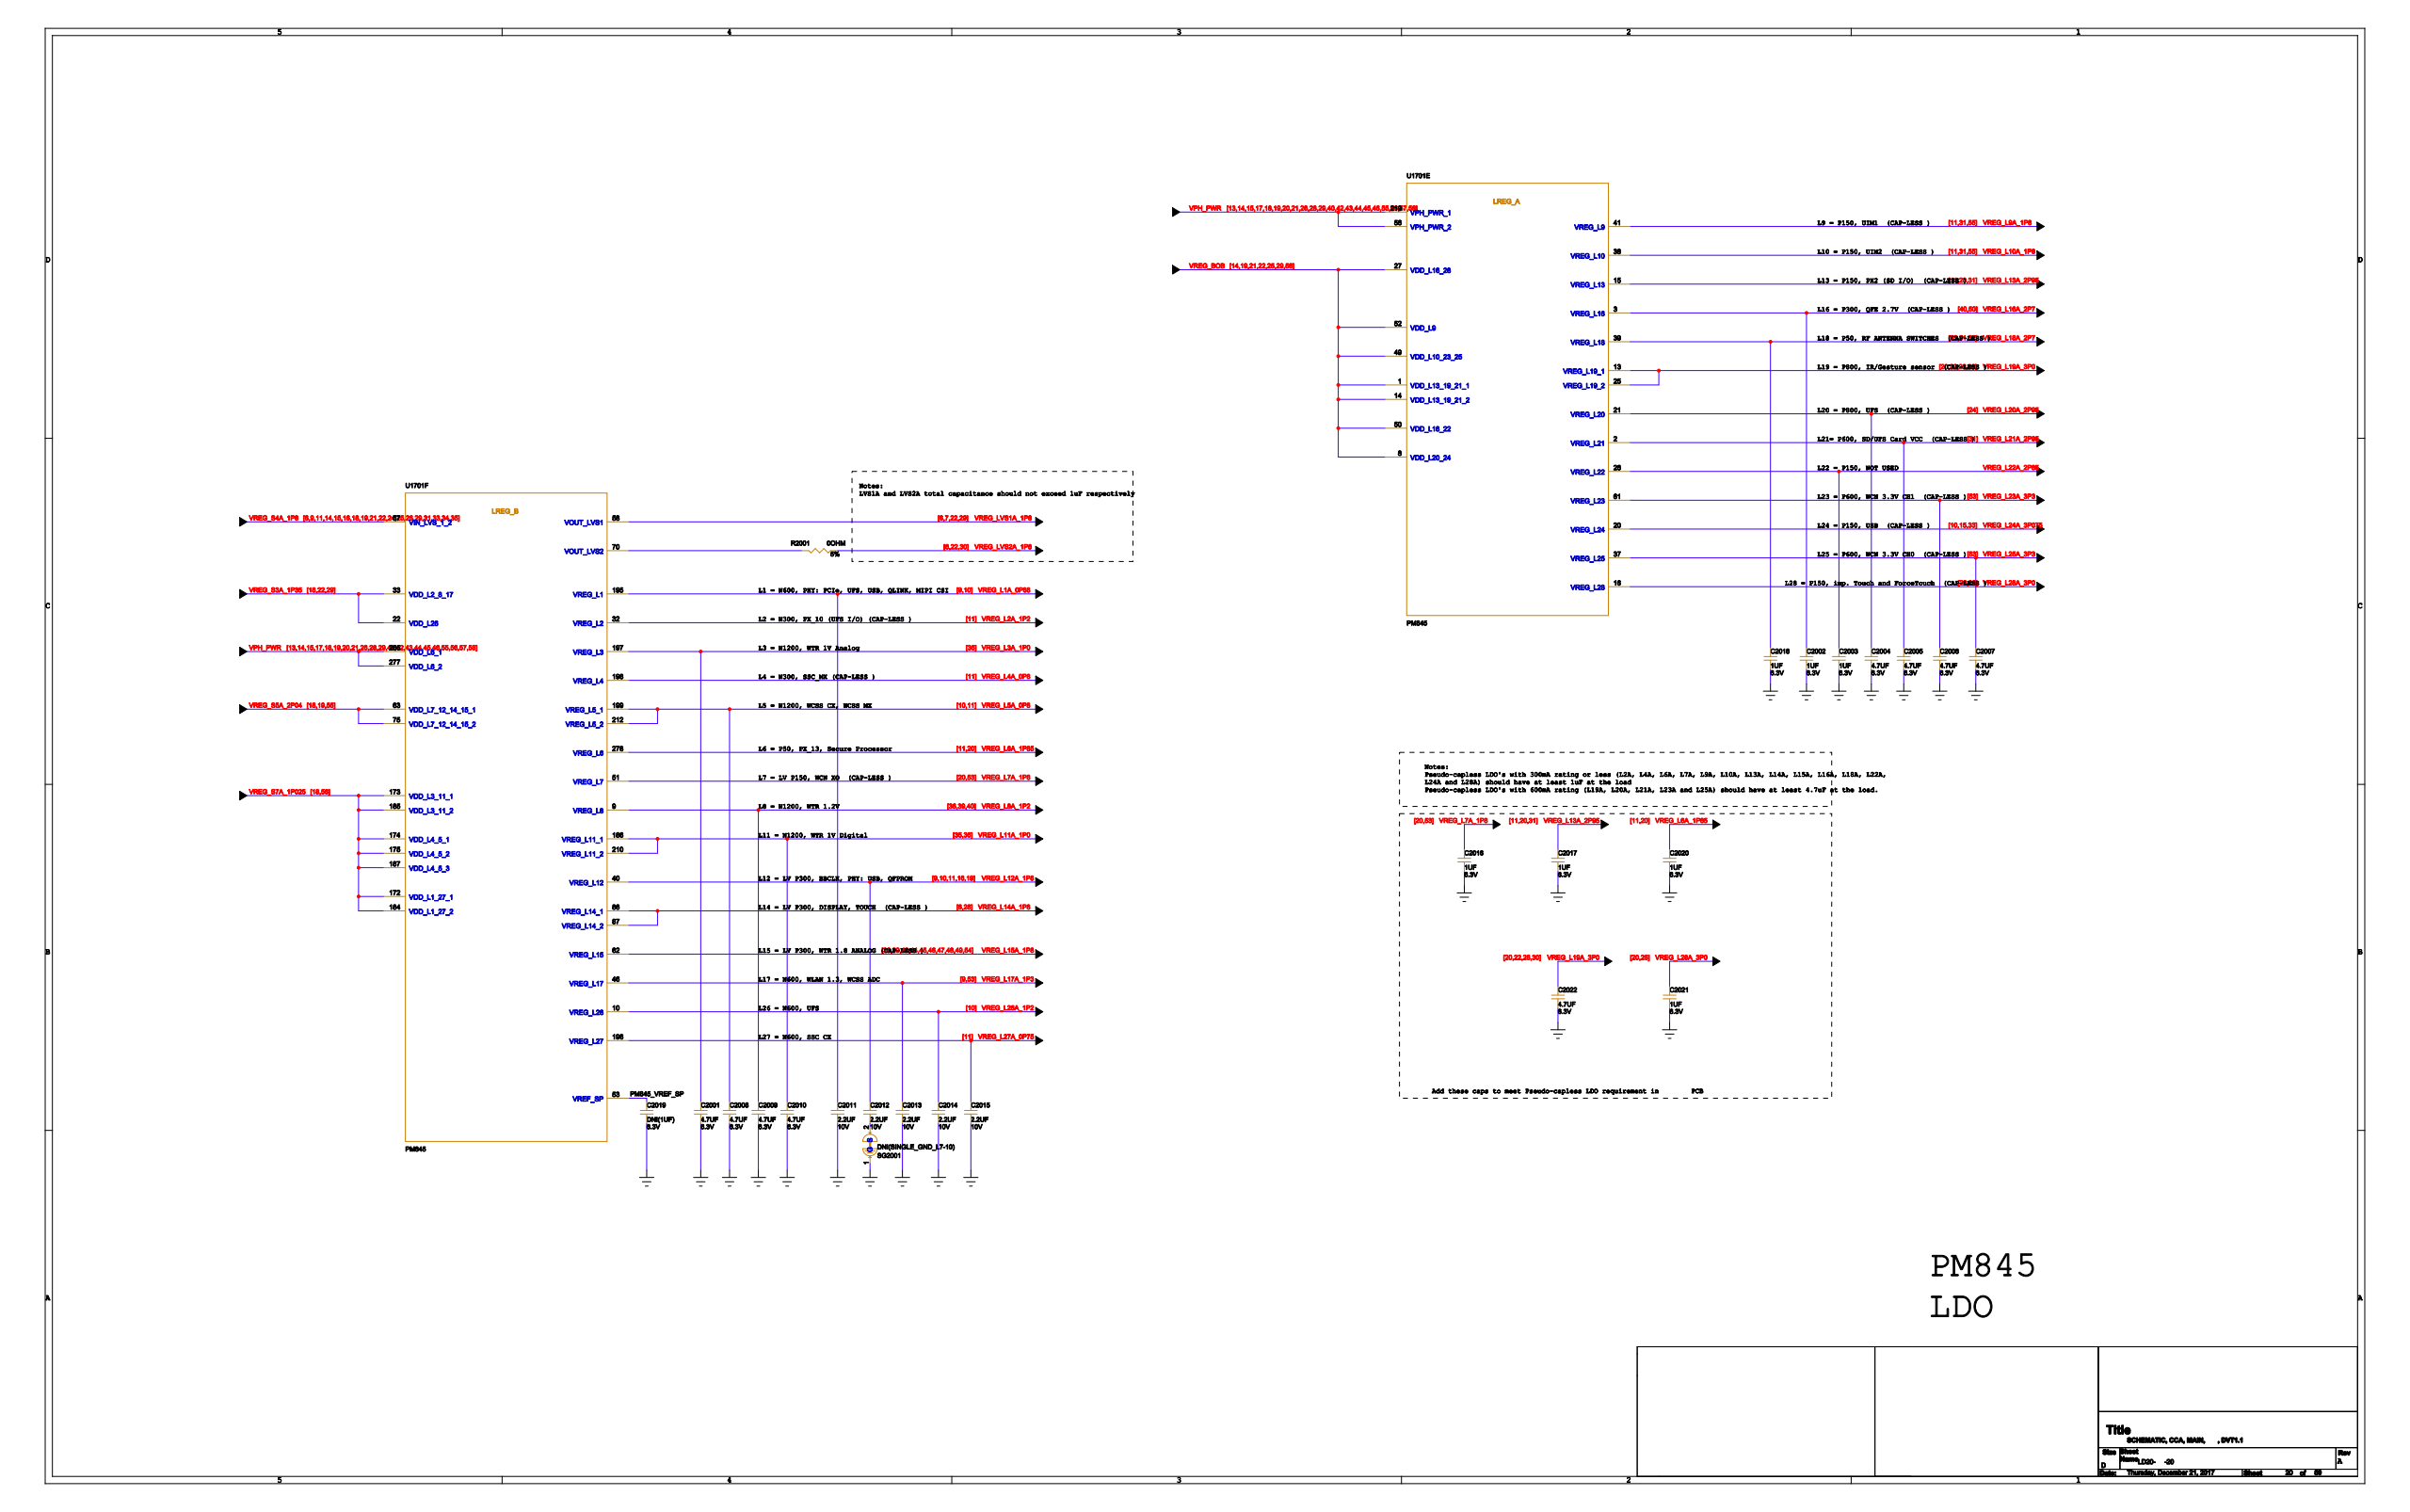Circuit board | Cadence Allegro | 1520 parts | 1149 nets | one sheet of the schematic
Parts on this sheet (reference | value | footprint):
C2001 | 4.7UF | 2P0402R
C2002 | 1UF | 2P0201R
C2003 | 1UF | 2P0201R
C2004 | 4.7UF | 2P0402R
C2005 | 4.7UF | 2P0402R
C2006 | 4.7UF | 2P0402R
C2007 | 4.7UF | 2P0402R
C2008 | 4.7UF | 2P0402R
C2009 | 4.7UF | 2P0402R
C2010 | 4.7UF | 2P0402R
C2011 | 2.2UF | 2P0402R
C2012 | 2.2UF | 2P0402R
C2013 | 2.2UF | 2P0402R
C2014 | 2.2UF | 2P0402R
C2015 | 2.2UF | 2P0402R
C2016 | 1UF | 2P0201R
C2017 | 1UF | 2P0201R
C2018 | 1UF | 2P0201R
C2019 | DNI(1UF) | 2P0201R_DNI
C2020 | 1UF | 2P0201R
C2021 | 1UF | 2P0201R
C2022 | 4.7UF | 2P0402R
R2001 | 0OHM | 2P0201R
SG2001 | DNI(SINGLE_GND_L7-10) | GND_L7-10
U1701 | PM845 | 287PGA242X240B138D45
Nets of these parts (net: part-pin ...):
GND: C2001-2 C2002-2 C2003-2 C2004-2 C2005-2 C2006-2 C2007-2 C2008-2 C2009-2 C2010-2 C2011-2 C2013-2 C2014-2 C2015-2 C2016-2 C2017-2 C2018-2 C2019-2 C2020-2 C2021-2 C2022-2 SG2001-1 U1701-7
VREG_BOB: U1701-1 U1701-8 U1701-14 U1701-27 U1701-49 U1701-50 U1701-52
VREG_S4A_1P8: U1701-57
VREG_L19A_3P0: C2022-1 U1701-13 U1701-25
VREG_LVS2A_1P8: R2001-2
N50935903: C2012-2 SG2001-2
VREG_S7A_1P025: U1701-172 U1701-173 U1701-174 U1701-175 U1701-184 U1701-185 U1701-187
VREG_S5A_2P04: U1701-29 U1701-63 U1701-75
VREG_L15A_1P8: U1701-62
VPH_PWR: U1701-48 U1701-56 U1701-219 U1701-265 U1701-277
VREG_S3A_1P35: U1701-22 U1701-33
VREG_LVS1A_1P8: U1701-58
VREG_L27A_0P75: C2015-1 U1701-196
VREG_L4A_0P8: U1701-198
VREG_L14A_1P8: U1701-86 U1701-87
VREG_L25A_3P3: C2007-1 U1701-37
PM845_VREF_SP: C2019-1 U1701-53
VREG_L24A_3P075: U1701-20
VREG_L9A_1P8: U1701-41
VREG_L10A_1P8: U1701-38
VREG_L12A_1P8: C2012-1 U1701-28 U1701-40
VREG_L11A_1P0: C2010-1 U1701-186 U1701-210
VREG_L3A_1P0: C2001-1 U1701-197
VREG_L8A_1P2: C2009-1 U1701-9
VREG_L16A_2P7: C2002-1 U1701-3
VREG_L20A_2P95: C2004-1 U1701-21
VREG_L6A_1P85: C2020-1 U1701-278
VREG_L28A_3P0: C2021-1 U1701-16
VREG_L17A_1P3: C2013-1 U1701-46
VREG_L1A_0P88: C2011-1 U1701-195
VREG_L26A_1P2: C2014-1 U1701-10
VREG_L5A_0P8: C2008-1 U1701-199 U1701-212
VREG_L13A_2P95: C2017-1 U1701-15
VREG_L2A_1P2: U1701-32
VREG_L22A_2P85: C2003-1 U1701-26
VREG_L7A_1P8: C2016-1 U1701-51
VREG_L18A_2P7: C2018-1 U1701-39
VREG_L21A_2P95: C2005-1 U1701-2
VREG_L23A_3P3: C2006-1 U1701-61
N34488142: R2001-1 U1701-70